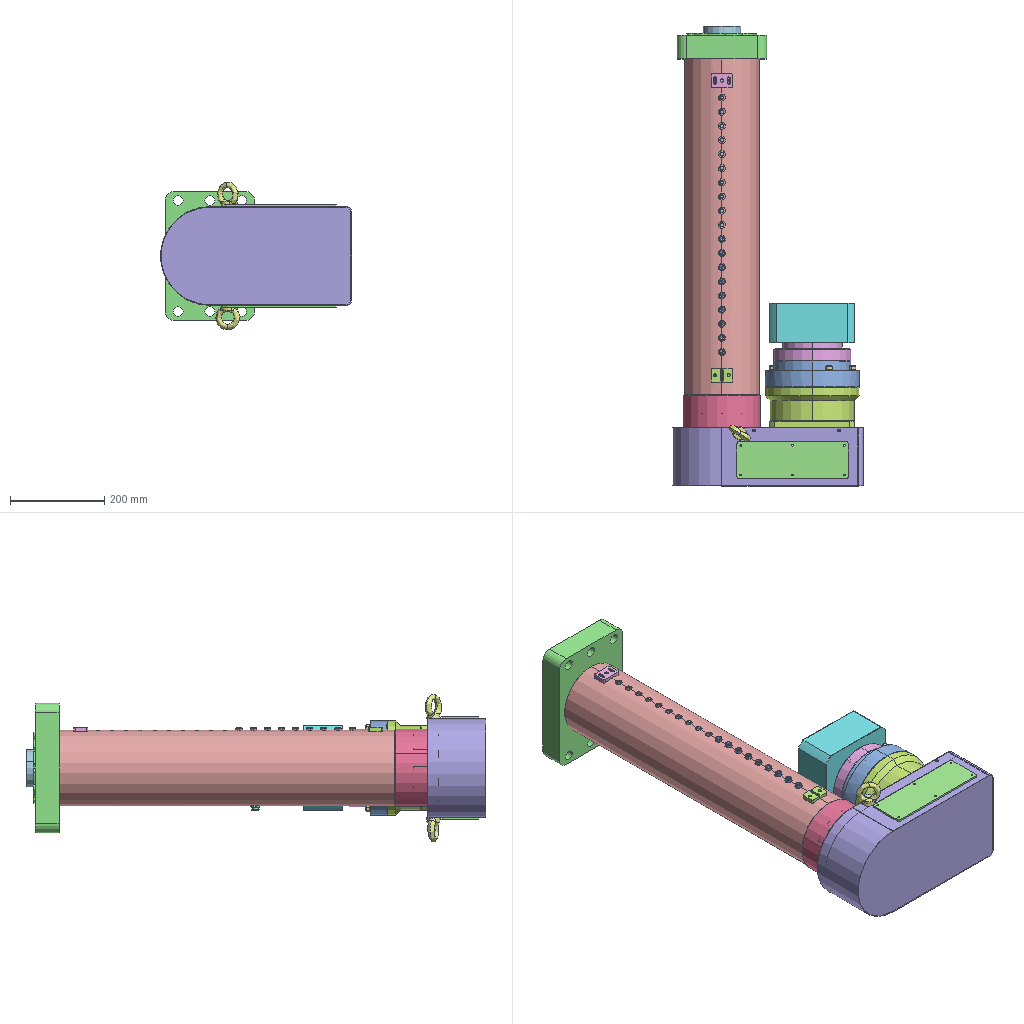Assembly | SolidWorks | 33 different items | 80 placed | box 404 x 976 x 313 mm
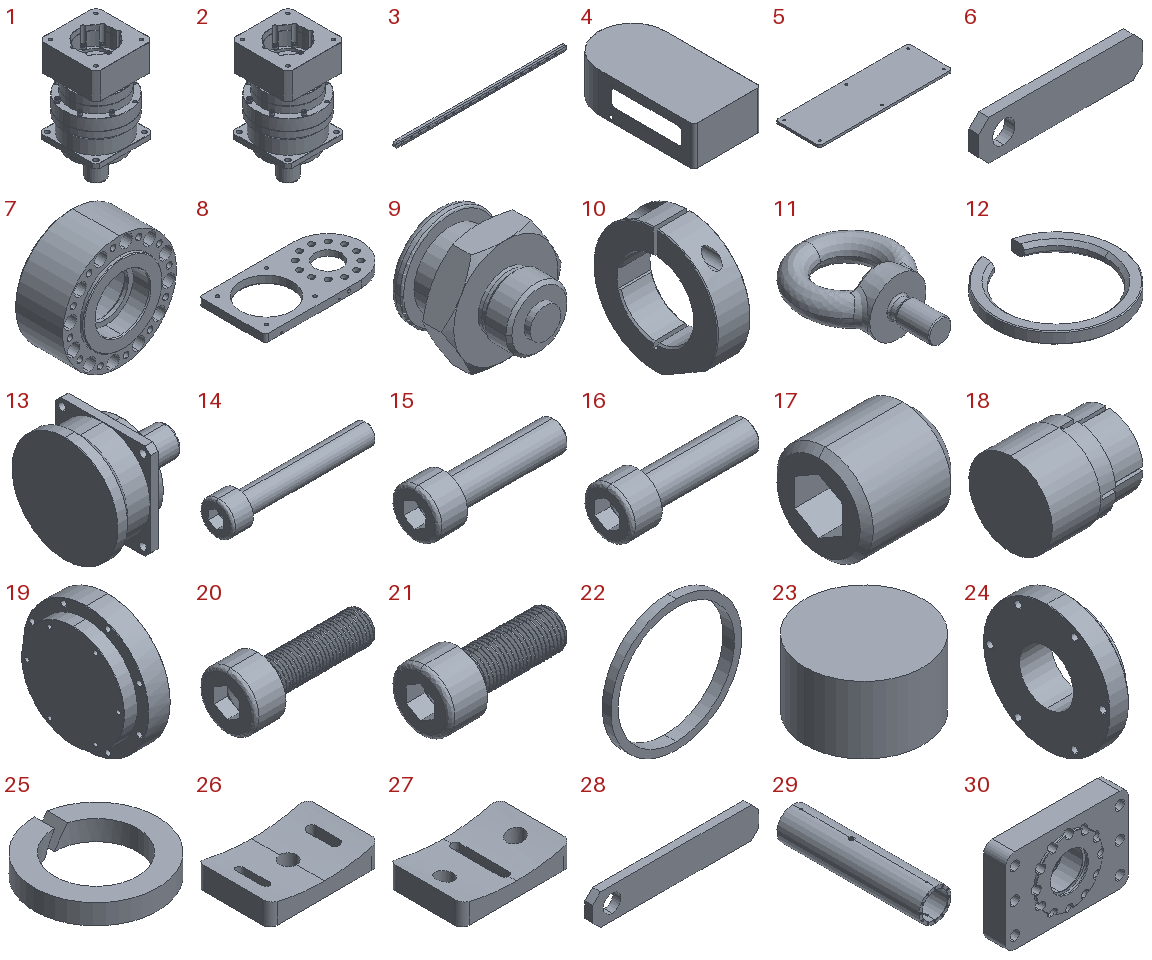Parts list (item | name | quantity | parent item | size | volume | features):
1 | (subassembly) | x1 | - | 200 x 200 x 369.495 mm | 7118058 mm3 | -
2 | (subassembly) | x1 | in 1 | 200 x 200 x 369.495 mm | 7118058 mm3 | -
3 | - | x1 | - | 605 x 9 x 20 mm | 97161 mm3 | features Chamfer 1, Extrusion 1, HoleWzd 1, ICE 1, LPattern 1
4 | - | x1 | - | 210 x 405 x 123 mm | 233905 mm3 | features ICE 5, Fillet 3, Extrusion 1
5 | - | x2 | - | 236 x 79 x 4 mm | 74259 mm3 | features Extrusion 1, Fillet 1, ICE 1
6 | - | x1 | - | 33 x 3 x 8 mm | 492.758 mm3 | features Chamfer 2, ICE 2, Extrusion 1
7 | - | x1 | - | 165 x 80.5 x 165 mm | 868351 mm3 | features ICE 9, Chamfer 7, HoleWzd 5, CirPattern 3, Extrusion 1, RefAxis 1
8 | - | x1 | - | 401.6 x 206.6 x 23 mm | 1126523 mm3 | features HoleWzd 6, ICE 3, MirrorPattern 3, Chamfer 2, CirPattern 1, Extrusion 1, Fillet 1
9 | - | x1 | - | 19.63 x 18 x 17 mm | 2444 mm3 | features BaseBody 1
10 | - | x1 | in 2 | 21 x 79 x 78.98 mm | 57883 mm3 | features BaseBody 1
11 | - | x2 | - | 52.011 x 73.603 x 29.1 mm | 21726 mm3 | features Fillet 5, Revolution 3, Chamfer 2, Blend 1, MirrorPattern 1
12 | - | x1 | - | 70 x 68.952 x 6.5 mm | 7783 mm3 | features Chamfer 2, Extrusion 1, ICE 1
13 | - | x1 | in 2 | 191.495 x 200 x 200 mm | 3024344 mm3 | features BaseBody 1
14 | - | x6 | in 2 | 58 x 13 x 13 mm | 3424 mm3 | features BaseBody 1
15 | - | x12 | in 2 | 38 x 13 x 13 mm | 2418 mm3 | features BaseBody 1
16 | - | x1 | in 2 | 45 x 16 x 16 mm | 4425 mm3 | features BaseBody 1
17 | - | x1 | in 2 | 16 x 16 x 16 mm | 2703 mm3 | features BaseBody 1
18 | - | x1 | in 2 | 64 x 55 x 55 mm | 51212 mm3 | features BaseBody 1
19 | - | x1 | in 2 | 56 x 200 x 200 mm | 1520895 mm3 | features BaseBody 1
20 | - | x4 | - | 13 x 5.5 x 5.5 mm | 124.477 mm3 | features BaseBody 1
21 | - | x9 | - | 28 x 13 x 13 mm | 1794 mm3 | features BaseBody 1
22 | - | x1 | - | 90 x 8 x 90 mm | 8779 mm3 | features Extrusion 1, ICE 1
23 | - | x2 | - | 8.8 x 8.8 x 5 mm | 304.106 mm3 | features Extrusion 1
24 | - | x1 | in 2 | 41 x 164 x 164 mm | 556620 mm3 | features BaseBody 1
25 | - | x18 | in 2 | 12.88 x 12.88 x 2.1 mm | 143.98 mm3 | features BaseBody 1
26 | - | x1 | - | 45 x 30 x 9.229 mm | 8297 mm3 | features ICE 2, Extrusion 1, Fillet 1, HoleWzd 1
27 | - | x1 | - | 45 x 30 x 9.229 mm | 8201 mm3 | features ICE 2, Extrusion 1, Fillet 1, HoleWzd 1
28 | - | x1 | - | 43 x 3 x 8 mm | 652.758 mm3 | features Chamfer 2, ICE 2, Extrusion 1
29 | - | x1 | - | 160 x 712.5 x 160 mm | 4794263 mm3 | features HoleWzd 5, ICE 5, Chamfer 2, MirrorPattern 2, CirPattern 1, Extrusion 1, LPattern 1
30 | - | x1 | - | 275 x 66 x 190 mm | 2101725 mm3 | features ICE 12, HoleWzd 3, Chamfer 2, CirPattern 2, MoveFace 2, Extrusion 1, Fillet 1
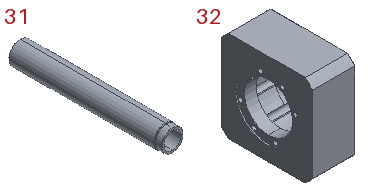31 | - | x1 | - | 80 x 534.5 x 80 mm | 1149532 mm3 | features ICE 8, Chamfer 7, HoleWzd 2, Extrusion 1, Fillet 1
32 | - | x1 | in 2 | 84 x 180 x 180 mm | 1847787 mm3 | features BaseBody 1
33 | hexagon socket head cap screws gb | x1 | - | - | - | -
Mates (type | each side: item.copy, entity, surface, feature):
Concentric | 31.1 face cylinder Boss-Extrude1 | assembly face
Coincident | 31.1 face plane Boss-Extrude1 | assembly face
Coincident | assembly face | assembly face | 23 times
Width | assembly face | assembly face | assembly face | assembly face | 4 times
Concentric | assembly face | assembly face | 18 times
DistanceDim | assembly face | assembly face
Concentric | 29.1 face cylinder Cut-Extrude2 | assembly face
Concentric | 29.1 face cylinder Cut-Extrude2 | 21.1 edge
Concentric | 29.1 face cylinder Boss-Extrude1 | 27.1 face cylinder Boss-Extrude1
Concentric | 29.1 face cylinder Boss-Extrude1 | 26.1 face cylinder Boss-Extrude1
Concentric | 29.1 face cylinder Boss-Extrude1 | 30.1 face cylinder Boss-Extrude2
Coincident | 29.1 face plane Boss-Extrude1 | 30.1 face plane Boss-Extrude1
Concentric | 29.1 face cylinder Boss-Extrude1 | 7.1 face cylinder Boss-Extrude2
Coincident | 29.1 face plane Boss-Extrude1 | 7.1 face plane Boss-Extrude1
Coincident | 29.1 face plane Cut-Extrude3 | 21.1 face plane Input1
Parallel | 27.1 face plane Boss-Extrude1 | 26.1 face plane Boss-Extrude1
Coincident | 27.1 face plane Cut-Extrude2 | 20.1 face plane Input1
Coincident | 27.1 face plane Cut-Extrude2 | 20.2 face plane Input1
Coincident | 26.1 face plane Cut-Extrude2 | 20.3 face plane Input1
Coincident | 26.1 face plane Cut-Extrude2 | 20.4 face plane Input1
Coincident | 22.1 face plane Boss-Extrude1 | 30.1 face plane Cut-Extrude3
Parallel | assembly face | assembly face | 8 times
Parallel | 30.1 face plane Boss-Extrude4 | assembly face | 3 times
Concentric | 7.1 face cylinder Boss-Extrude2 | assembly face | 2 times
Coincident | 7.1 face plane Boss-Extrude2 | assembly face | 2 times
Concentric | 27.1 face cylinder M8x1.0 Tapped Hole1 | assembly face | 2 times
Coincident | 27.1 face plane Boss-Extrude1 | assembly face
Concentric | 26.1 face cylinder M8x1.0 Tapped Hole1 | assembly face | 2 times
Coincident | 26.1 face plane Boss-Extrude1 | assembly face | 2 times
Concentric | 7.1 face cylinder Boss-Extrude3 | assembly face
Concentric | 7.1 face cylinder CirPattern3 | assembly face
Coincident | 7.1 face plane Boss-Extrude1 | assembly face | 2 times
Concentric | 11.1 face cylinder Revolve3 | assembly edge
Coincident | 11.1 face plane Revolve1 | assembly face | 2 times
Concentric | 11.2 face cylinder Revolve3 | assembly face
Coincident | 11.2 face plane Revolve1 | assembly face
Concentric | assembly face | assembly edge
Slot | 27.1 face cylinder M8x1.0 Tapped Hole1 | 29.1 face cylinder Cut-Extrude12
Tangent | 29.1 face cylinder Boss-Extrude1 | assembly face
Slot | 26.1 face cylinder M8x1.0 Tapped Hole1 | 29.1 face cylinder Cut-Extrude13
Parallel | 27.1 face plane Boss-Extrude1 | assembly face
Concentric | 22.1 face cylinder Boss-Extrude1 | 31.1 face cylinder Boss-Extrude1
Coincident | 30.1 face plane Boss-Extrude1 | assembly face
Coincident | 30.1 face plane Boss-Extrude4 | assembly face
Concentric | 7.1 face cylinder Boss-Extrude3 | 8.1 face cylinder Cut-Extrude3
Parallel | assembly face | 8.1 face plane Boss-Extrude1 | 2 times
Coincident | 7.1 face plane Boss-Extrude1 | 8.1 face plane Boss-Extrude1
Concentric | 8.1 face cylinder Cut-Extrude1 | 13.1 face cylinder Input1
Parallel | 8.1 face plane Boss-Extrude1 | 13.1 face plane Input1
Coincident | 8.1 face plane Boss-Extrude1 | 13.1 face plane Input1
Concentric | 13.1 face cylinder Input1 | 12.1 edge
Coincident | 13.1 face plane Input1 | 12.1 face plane Boss-Extrude1
Concentric | assembly face | 8.1 face cylinder Boss-Extrude1
Coincident | assembly face | 8.1 face plane Boss-Extrude1
Concentric | 29.1 face cylinder M3 Tapped Hole4 | 20.1 face cone Input1
Concentric | 29.1 face cylinder M3 Tapped Hole4 | 20.2 face cone Input1
Concentric | 29.1 face cylinder M10x1.0 Tapped Hole1 | 9.1 face cylinder Input1
Coincident | 29.1 face plane Cut-Extrude14 | 9.1 face plane Input1
Concentric | 29.1 face cylinder G1/8 Tapped Hole2 | 23.1 face cylinder Boss-Extrude1
Tangent | 29.1 face cylinder Boss-Extrude1 | 23.1 face plane Boss-Extrude1
Concentric | 29.1 face cylinder G1/8 Tapped Hole2 | 23.2 face cylinder Boss-Extrude1
Tangent | 29.1 face cylinder Boss-Extrude1 | 23.2 face plane Boss-Extrude1
Parallel | assembly face | assembly plane
Concentric | 11.1 face cylinder Revolve3 | 8.1 face cylinder Mirror5
Tangent | 29.1 face cylinder Boss-Extrude1 | 3.1 face plane Boss-Extrude1
Concentric | 8.1 face cylinder M12 Tapped Hole3 | 4.1 face cylinder Cut-Extrude2
Concentric | 8.1 face cylinder Boss-Extrude1 | 4.1 face cylinder Boss-Extrude1
Coincident | 8.1 face plane Boss-Extrude1 | 4.1 face plane Boss-Extrude1
Concentric | 4.1 face cylinder Cut-Extrude4 | 5.1 face cylinder Cut-Extrude1 | 2 times
Coincident | 4.1 face plane Boss-Extrude1 | 5.1 face plane Boss-Extrude1
Parallel | 4.1 face plane Boss-Extrude1 | assembly plane
Concentric | 4.1 face cylinder Cut-Extrude4 | 5.2 face cylinder Cut-Extrude1
Coincident | 4.1 face cylinder Cut-Extrude4 | 5.2 edge
Coincident | 4.1 face plane Boss-Extrude1 | 5.2 face plane Boss-Extrude1
Coincident | 11.1 face plane Revolve1 | 4.1 face plane Boss-Extrude1
Concentric | 29.1 face cylinder M3 Tapped Hole5 | 20.4 face cylinder Input1
Concentric | 29.1 face cylinder M3 Tapped Hole5 | 20.3 face cylinder Input1
Concentric | 11.2 face cylinder Revolve3 | 8.1 face cylinder M12 Tapped Hole3
Coincident | 11.2 face plane Revolve1 | 4.1 face plane Boss-Extrude1
Concentric | 29.1 face cylinder Mirror2 | 30.1 face cylinder CirPattern1 | 2 times
Concentric | 29.1 face cylinder LPattern1 | 3.1 face cylinder M8 Tapped Hole1
Concentric | 29.1 face cylinder Cut-Extrude2 | 3.1 face cylinder LPattern1
Parallel | 30.1 face plane Boss-Extrude4 | 4.1 face plane Boss-Extrude1